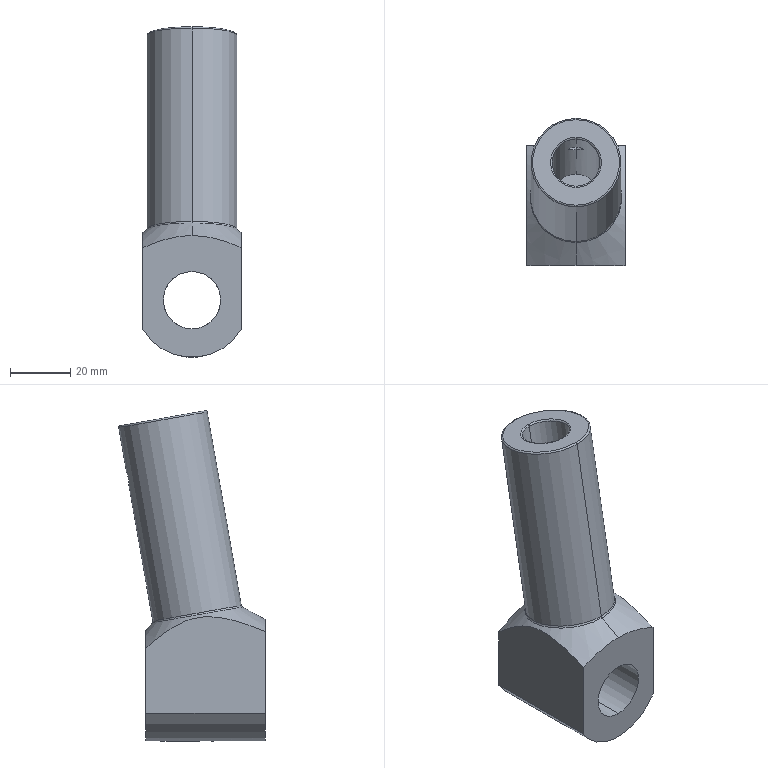Part | SolidWorks | features ICE 6, Fillet 2, 3DProfileFeature 1, Extrusion 1, HoleWzd 1, RevCutThin 1 | 1 solid | 27 faces | box 32.614 x 48.684 x 109.683 mm | volume 70811 mm3 | cylinder 12 | plane 7 | torus 6 | cone 2 | commonest cylinder face diameters 4.762 x2 5.41 x2 15.888 x2 19.05 x2 29.845 x2 15.875 x1
STEP:
#1=CARTESIAN_POINT('',(0.,1.053,2.59));
#2=VERTEX_POINT('',#1);
#3=CARTESIAN_POINT('',(0.,1.086,2.774));
#4=VERTEX_POINT('',#3);
#5=CARTESIAN_POINT('',(0.,1.053,2.59));
#6=CARTESIAN_POINT('',(-0.006205,1.053,2.59));
#7=CARTESIAN_POINT('',(-0.0123,1.053,2.59));
#8=CARTESIAN_POINT('',(-0.0243,1.053,2.593));
#9=CARTESIAN_POINT('',(-0.03026,1.053,2.595));
#10=CARTESIAN_POINT('',(-0.04161,1.053,2.599));
#11=CARTESIAN_POINT('',(-0.04699,1.054,2.602));
#12=CARTESIAN_POINT('',(-0.05718,1.054,2.609));
#13=CARTESIAN_POINT('',(-0.06199,1.054,2.613));
#14=CARTESIAN_POINT('',(-0.07494,1.055,2.626));
#15=CARTESIAN_POINT('',(-0.08192,1.056,2.637));
#16=CARTESIAN_POINT('',(-0.08894,1.058,2.653));
#17=CARTESIAN_POINT('',(-0.09074,1.058,2.659));
#18=CARTESIAN_POINT('',(-0.09315,1.06,2.671));
#19=CARTESIAN_POINT('',(-0.09375,1.061,2.677));
#20=CARTESIAN_POINT('',(-0.09375,1.063,2.689));
#21=CARTESIAN_POINT('',(-0.09314,1.064,2.696));
#22=CARTESIAN_POINT('',(-0.09074,1.067,2.707));
#23=CARTESIAN_POINT('',(-0.08897,1.068,2.713));
#24=CARTESIAN_POINT('',(-0.08426,1.071,2.724));
#25=CARTESIAN_POINT('',(-0.08133,1.072,2.729));
#26=CARTESIAN_POINT('',(-0.07454,1.075,2.739));
#27=CARTESIAN_POINT('',(-0.07066,1.076,2.744));
#28=CARTESIAN_POINT('',(-0.06193,1.079,2.752));
#29=CARTESIAN_POINT('',(-0.0572,1.08,2.756));
#30=CARTESIAN_POINT('',(-0.04706,1.082,2.763));
#31=CARTESIAN_POINT('',(-0.04157,1.083,2.765));
#32=CARTESIAN_POINT('',(-0.03023,1.084,2.77));
#33=CARTESIAN_POINT('',(-0.02438,1.085,2.772));
#34=CARTESIAN_POINT('',(-0.01234,1.086,2.774));
#35=CARTESIAN_POINT('',(-0.006124,1.086,2.774));
#36=CARTESIAN_POINT('',(0.,1.086,2.774));
#37=B_SPLINE_CURVE_WITH_KNOTS('',3,(#5,#6,#7,#8,#9,#10,#11,#12,#13,#14,#15,#16,#17,#18,#19,#20,#21,#22,#23,#24,#25,#26,#27,#28,#29,#30,#31,#32,#33,#34,#35,#36),.UNSPECIFIED.,.F.,.F.,(4,2,2,2,2,2,2,2,2,2,2,2,2,2,2,4),(0.,0.000466,0.0009321,0.001398,0.001864,0.002796,0.003262,0.003728,0.004194,0.00466,0.005127,0.005593,0.006059,0.006525,0.006991,0.007457),.UNSPECIFIED.);
#38=EDGE_CURVE('',#2,#4,#37,.T.);
#39=ORIENTED_EDGE('',*,*,#38,.T.);
#40=CARTESIAN_POINT('',(0.,0.8152,2.822));
#41=VERTEX_POINT('',#40);
#42=CARTESIAN_POINT('',(0.,3.094,2.42));
#43=DIRECTION('',(0.,-0.9848,0.1736));
#44=VECTOR('',#43,39.37);
#45=LINE('',#42,#44);
#46=EDGE_CURVE('',#4,#41,#45,.T.);
#47=ORIENTED_EDGE('',*,*,#46,.T.);
#48=CARTESIAN_POINT('',(0.,0.7826,2.637));
#49=VERTEX_POINT('',#48);
#50=CARTESIAN_POINT('',(0.,0.7826,2.637));
#51=CARTESIAN_POINT('',(-0.006233,0.7826,2.637));
#52=CARTESIAN_POINT('',(-0.01235,0.7826,2.638));
#53=CARTESIAN_POINT('',(-0.02439,0.7823,2.641));
#54=CARTESIAN_POINT('',(-0.03036,0.7821,2.642));
#55=CARTESIAN_POINT('',(-0.0417,0.7816,2.647));
#56=CARTESIAN_POINT('',(-0.04707,0.7813,2.65));
#57=CARTESIAN_POINT('',(-0.05724,0.7808,2.657));
#58=CARTESIAN_POINT('',(-0.06202,0.7806,2.661));
#59=CARTESIAN_POINT('',(-0.07491,0.7801,2.675));
#60=CARTESIAN_POINT('',(-0.08188,0.78,2.685));
#61=CARTESIAN_POINT('',(-0.0889,0.7809,2.702));
#62=CARTESIAN_POINT('',(-0.09072,0.7814,2.708));
#63=CARTESIAN_POINT('',(-0.09314,0.7828,2.72));
#64=CARTESIAN_POINT('',(-0.09375,0.7837,2.726));
#65=CARTESIAN_POINT('',(-0.09375,0.7858,2.738));
#66=CARTESIAN_POINT('',(-0.09313,0.7871,2.744));
#67=CARTESIAN_POINT('',(-0.09072,0.7899,2.756));
#68=CARTESIAN_POINT('',(-0.08894,0.7915,2.762));
#69=CARTESIAN_POINT('',(-0.08183,0.7964,2.778));
#70=CARTESIAN_POINT('',(-0.07493,0.8001,2.788));
#71=CARTESIAN_POINT('',(-0.06194,0.8051,2.8));
#72=CARTESIAN_POINT('',(-0.05725,0.8067,2.804));
#73=CARTESIAN_POINT('',(-0.04711,0.8096,2.81));
#74=CARTESIAN_POINT('',(-0.04162,0.8109,2.813));
#75=CARTESIAN_POINT('',(-0.03032,0.813,2.818));
#76=CARTESIAN_POINT('',(-0.02447,0.8138,2.819));
#77=CARTESIAN_POINT('',(-0.01236,0.8149,2.822));
#78=CARTESIAN_POINT('',(-0.006142,0.8152,2.822));
#79=CARTESIAN_POINT('',(0.,0.8152,2.822));
#80=B_SPLINE_CURVE_WITH_KNOTS('',3,(#50,#51,#52,#53,#54,#55,#56,#57,#58,#59,#60,#61,#62,#63,#64,#65,#66,#67,#68,#69,#70,#71,#72,#73,#74,#75,#76,#77,#78,#79),.UNSPECIFIED.,.F.,.F.,(4,2,2,2,2,2,2,2,2,2,2,2,2,2,4),(0.,0.000468,0.000936,0.001404,0.001872,0.002808,0.003276,0.003744,0.004212,0.00468,0.005616,0.006084,0.006552,0.00702,0.007488),.UNSPECIFIED.);
#81=EDGE_CURVE('',#49,#41,#80,.T.);
#82=ORIENTED_EDGE('',*,*,#81,.F.);
#83=CARTESIAN_POINT('',(0.,3.062,2.236));
#84=DIRECTION('',(0.,-0.9848,0.1736));
#85=VECTOR('',#84,39.37);
#86=LINE('',#83,#85);
#87=EDGE_CURVE('',#2,#49,#86,.T.);
#88=ORIENTED_EDGE('',*,*,#87,.F.);
#89=EDGE_LOOP('',(#39,#47,#82,#88));
#90=FACE_OUTER_BOUND('',#89,.T.);
#91=CARTESIAN_POINT('',(0.,3.078,2.328));
#92=DIRECTION('',(0.,-0.9848,0.1736));
#93=DIRECTION('',(0.,-0.1736,-0.9848));
#94=AXIS2_PLACEMENT_3D('',#91,#92,#93);
#95=CYLINDRICAL_SURFACE('',#94,0.09375);
#96=ADVANCED_FACE('',(#90),#95,.F.);
#97=CARTESIAN_POINT('',(0.1065,0.05244,-0.3596));
#98=VERTEX_POINT('',#97);
#99=CARTESIAN_POINT('',(0.,-0.05406,-0.375));
#100=VERTEX_POINT('',#99);
#101=CARTESIAN_POINT('',(0.1065,0.05244,-0.3596));
#102=CARTESIAN_POINT('',(0.1065,0.0385,-0.3596));
#103=CARTESIAN_POINT('',(0.1037,0.02442,-0.3604));
#104=CARTESIAN_POINT('',(0.09569,0.005169,-0.3626));
#105=CARTESIAN_POINT('',(0.09235,-0.001061,-0.3635));
#106=CARTESIAN_POINT('',(0.08462,-0.01259,-0.3653));
#107=CARTESIAN_POINT('',(0.08024,-0.01793,-0.3663));
#108=CARTESIAN_POINT('',(0.07042,-0.02776,-0.3684));
#109=CARTESIAN_POINT('',(0.06499,-0.03222,-0.3694));
#110=CARTESIAN_POINT('',(0.0535,-0.03991,-0.3712));
#111=CARTESIAN_POINT('',(0.04739,-0.04319,-0.3721));
#112=CARTESIAN_POINT('',(0.0344,-0.04859,-0.3735));
#113=CARTESIAN_POINT('',(0.02773,-0.05062,-0.374));
#114=CARTESIAN_POINT('',(0.01408,-0.05335,-0.3748));
#115=CARTESIAN_POINT('',(0.007021,-0.05406,-0.375));
#116=CARTESIAN_POINT('',(0.,-0.05406,-0.375));
#117=B_SPLINE_CURVE_WITH_KNOTS('',3,(#101,#102,#103,#104,#105,#106,#107,#108,#109,#110,#111,#112,#113,#114,#115,#116),.UNSPECIFIED.,.F.,.F.,(4,2,2,2,2,2,2,4),(0.008501,0.009564,0.01009,0.01063,0.01116,0.01169,0.01222,0.01275),.UNSPECIFIED.);
#118=EDGE_CURVE('',#98,#100,#117,.T.);
#119=ORIENTED_EDGE('',*,*,#118,.F.);
#120=CARTESIAN_POINT('',(0.1065,0.05244,-0.7383));
#121=VERTEX_POINT('',#120);
#122=CARTESIAN_POINT('',(0.1065,0.05244,-0.7459));
#123=DIRECTION('',(0.,0.,-1.));
#124=VECTOR('',#123,39.37);
#125=LINE('',#122,#124);
#126=EDGE_CURVE('',#98,#121,#125,.T.);
#127=ORIENTED_EDGE('',*,*,#126,.T.);
#128=CARTESIAN_POINT('',(-0.1065,0.05244,-0.7383));
#129=VERTEX_POINT('',#128);
#130=CARTESIAN_POINT('',(-0.1065,0.05244,-0.7383));
#131=CARTESIAN_POINT('',(-0.1065,0.0454,-0.7383));
#132=CARTESIAN_POINT('',(-0.1058,0.03847,-0.7384));
#133=CARTESIAN_POINT('',(-0.1031,0.02484,-0.7387));
#134=CARTESIAN_POINT('',(-0.101,0.01807,-0.739));
#135=CARTESIAN_POINT('',(-0.09569,0.00518,-0.7397));
#136=CARTESIAN_POINT('',(-0.09242,-0.0009336,-0.7402));
#137=CARTESIAN_POINT('',(-0.08469,-0.0125,-0.7411));
#138=CARTESIAN_POINT('',(-0.0802,-0.01798,-0.7416));
#139=CARTESIAN_POINT('',(-0.07038,-0.02779,-0.7426));
#140=CARTESIAN_POINT('',(-0.06503,-0.03219,-0.7431));
#141=CARTESIAN_POINT('',(-0.05339,-0.03998,-0.744));
#142=CARTESIAN_POINT('',(-0.0472,-0.04328,-0.7444));
#143=CARTESIAN_POINT('',(-0.03439,-0.04859,-0.7451));
#144=CARTESIAN_POINT('',(-0.02767,-0.05064,-0.7454));
#145=CARTESIAN_POINT('',(-0.01391,-0.05338,-0.7458));
#146=CARTESIAN_POINT('',(-0.006996,-0.05406,-0.7459));
#147=CARTESIAN_POINT('',(0.006917,-0.05406,-0.7459));
#148=CARTESIAN_POINT('',(0.01398,-0.05337,-0.7458));
#149=CARTESIAN_POINT('',(0.02765,-0.05064,-0.7454));
#150=CARTESIAN_POINT('',(0.03429,-0.04863,-0.7451));
#151=CARTESIAN_POINT('',(0.0472,-0.04328,-0.7444));
#152=CARTESIAN_POINT('',(0.05342,-0.03995,-0.744));
#153=CARTESIAN_POINT('',(0.06495,-0.03224,-0.7431));
#154=CARTESIAN_POINT('',(0.07034,-0.02783,-0.7426));
#155=CARTESIAN_POINT('',(0.08027,-0.01791,-0.7416));
#156=CARTESIAN_POINT('',(0.08467,-0.01253,-0.7411));
#157=CARTESIAN_POINT('',(0.09238,-0.001008,-0.7402));
#158=CARTESIAN_POINT('',(0.09572,0.005224,-0.7397));
#159=CARTESIAN_POINT('',(0.1011,0.01811,-0.739));
#160=CARTESIAN_POINT('',(0.1031,0.02475,-0.7387));
#161=CARTESIAN_POINT('',(0.1058,0.03842,-0.7384));
#162=CARTESIAN_POINT('',(0.1065,0.04549,-0.7383));
#163=CARTESIAN_POINT('',(0.1065,0.05244,-0.7383));
#164=B_SPLINE_CURVE_WITH_KNOTS('',3,(#130,#131,#132,#133,#134,#135,#136,#137,#138,#139,#140,#141,#142,#143,#144,#145,#146,#147,#148,#149,#150,#151,#152,#153,#154,#155,#156,#157,#158,#159,#160,#161,#162,#163),.UNSPECIFIED.,.F.,.F.,(4,2,2,2,2,2,2,2,2,2,2,2,2,2,2,2,4),(0.,0.0005293,0.001059,0.001588,0.002117,0.002646,0.003176,0.003705,0.004234,0.004763,0.005293,0.005822,0.006351,0.00688,0.00741,0.007939,0.008468),.UNSPECIFIED.);
#165=EDGE_CURVE('',#129,#121,#164,.T.);
#166=ORIENTED_EDGE('',*,*,#165,.F.);
#167=CARTESIAN_POINT('',(-0.1065,0.05244,-0.3596));
#168=VERTEX_POINT('',#167);
#169=CARTESIAN_POINT('',(-0.1065,0.05244,-0.7459));
#170=DIRECTION('',(0.,0.,-1.));
#171=VECTOR('',#170,39.37);
#172=LINE('',#169,#171);
#173=EDGE_CURVE('',#168,#129,#172,.T.);
#174=ORIENTED_EDGE('',*,*,#173,.F.);
#175=CARTESIAN_POINT('',(0.,-0.05406,-0.375));
#176=CARTESIAN_POINT('',(-0.00702,-0.05406,-0.375));
#177=CARTESIAN_POINT('',(-0.01396,-0.05337,-0.3748));
#178=CARTESIAN_POINT('',(-0.02766,-0.05064,-0.374));
#179=CARTESIAN_POINT('',(-0.03446,-0.04857,-0.3735));
#180=CARTESIAN_POINT('',(-0.05371,-0.04057,-0.3714));
#181=CARTESIAN_POINT('',(-0.06552,-0.03265,-0.3694));
#182=CARTESIAN_POINT('',(-0.08017,-0.018,-0.3664));
#183=CARTESIAN_POINT('',(-0.08463,-0.01258,-0.3653));
#184=CARTESIAN_POINT('',(-0.09237,-0.00102,-0.3635));
#185=CARTESIAN_POINT('',(-0.09564,0.005076,-0.3626));
#186=CARTESIAN_POINT('',(-0.101,0.01791,-0.3612));
#187=CARTESIAN_POINT('',(-0.1031,0.0247,-0.3606));
#188=CARTESIAN_POINT('',(-0.1058,0.03841,-0.3598));
#189=CARTESIAN_POINT('',(-0.1065,0.04537,-0.3596));
#190=CARTESIAN_POINT('',(-0.1065,0.05244,-0.3596));
#191=B_SPLINE_CURVE_WITH_KNOTS('',3,(#175,#176,#177,#178,#179,#180,#181,#182,#183,#184,#185,#186,#187,#188,#189,#190),.UNSPECIFIED.,.F.,.F.,(4,2,2,2,2,2,2,4),(0.01275,0.01328,0.01381,0.01488,0.01541,0.01594,0.01647,0.017),.UNSPECIFIED.);
#192=EDGE_CURVE('',#100,#168,#191,.T.);
#193=ORIENTED_EDGE('',*,*,#192,.F.);
#194=EDGE_LOOP('',(#119,#127,#166,#174,#193));
#195=FACE_OUTER_BOUND('',#194,.T.);
#196=CARTESIAN_POINT('',(0.,0.05244,-0.7459));
#197=DIRECTION('',(0.,0.,-1.));
#198=DIRECTION('',(-1.,0.,0.));
#199=AXIS2_PLACEMENT_3D('',#196,#197,#198);
#200=CYLINDRICAL_SURFACE('',#199,0.1065);
#201=ADVANCED_FACE('',(#195),#200,.F.);
#202=CARTESIAN_POINT('',(0.,0.301,3.508));
#203=VERTEX_POINT('',#202);
#204=CARTESIAN_POINT('',(0.,0.917,3.399));
#205=VERTEX_POINT('',#204);
#206=CARTESIAN_POINT('',(0.,0.609,3.454));
#207=DIRECTION('',(0.,0.1736,0.9848));
#208=DIRECTION('',(0.,0.9848,-0.1736));
#209=AXIS2_PLACEMENT_3D('',#206,#207,#208);
#210=CIRCLE('',#209,0.3128);
#211=EDGE_CURVE('',#203,#205,#210,.T.);
#212=ORIENTED_EDGE('',*,*,#211,.F.);
#213=CARTESIAN_POINT('',(0.,0.2848,3.531));
#214=VERTEX_POINT('',#213);
#215=CARTESIAN_POINT('',(0.,0.2813,3.512));
#216=DIRECTION('',(1.,0.,0.));
#217=DIRECTION('',(0.,1.,0.));
#218=AXIS2_PLACEMENT_3D('',#215,#216,#217);
#219=CIRCLE('',#218,0.02);
#220=EDGE_CURVE('',#203,#214,#219,.T.);
#221=ORIENTED_EDGE('',*,*,#220,.T.);
#222=CARTESIAN_POINT('',(0.,0.9402,3.416));
#223=VERTEX_POINT('',#222);
#224=CARTESIAN_POINT('',(0.,0.6125,3.473));
#225=DIRECTION('',(0.,-0.1736,-0.9848));
#226=DIRECTION('',(0.,0.9848,-0.1736));
#227=AXIS2_PLACEMENT_3D('',#224,#225,#226);
#228=CIRCLE('',#227,0.3327);
#229=EDGE_CURVE('',#223,#214,#228,.T.);
#230=ORIENTED_EDGE('',*,*,#229,.F.);
#231=CARTESIAN_POINT('',(0.,0.9367,3.396));
#232=DIRECTION('',(-1.,0.,0.));
#233=DIRECTION('',(0.,0.,1.));
#234=AXIS2_PLACEMENT_3D('',#231,#232,#233);
#235=CIRCLE('',#234,0.02);
#236=EDGE_CURVE('',#205,#223,#235,.T.);
#237=ORIENTED_EDGE('',*,*,#236,.F.);
#238=EDGE_LOOP('',(#212,#221,#230,#237));
#239=FACE_OUTER_BOUND('',#238,.T.);
#240=CARTESIAN_POINT('',(0.,0.609,3.454));
#241=DIRECTION('',(0.,-0.1736,-0.9848));
#242=DIRECTION('',(0.,0.9848,-0.1736));
#243=AXIS2_PLACEMENT_3D('',#240,#241,#242);
#244=TOROIDAL_SURFACE('',#243,0.3327,0.02);
#245=ADVANCED_FACE('',(#239),#244,.T.);
#246=CARTESIAN_POINT('',(0.,0.05359,3.572));
#247=VERTEX_POINT('',#246);
#248=CARTESIAN_POINT('',(0.,1.171,3.375));
#249=VERTEX_POINT('',#248);
#250=CARTESIAN_POINT('',(0.,0.6125,3.473));
#251=DIRECTION('',(0.,0.1736,0.9848));
#252=DIRECTION('',(0.,0.9848,-0.1736));
#253=AXIS2_PLACEMENT_3D('',#250,#251,#252);
#254=CIRCLE('',#253,0.5675);
#255=EDGE_CURVE('',#247,#249,#254,.T.);
#256=ORIENTED_EDGE('',*,*,#255,.F.);
#257=CARTESIAN_POINT('',(0.,0.03042,3.556));
#258=VERTEX_POINT('',#257);
#259=CARTESIAN_POINT('',(0.,0.05012,3.552));
#260=DIRECTION('',(1.,0.,0.));
#261=DIRECTION('',(0.,1.,0.));
#262=AXIS2_PLACEMENT_3D('',#259,#260,#261);
#263=CIRCLE('',#262,0.02);
#264=EDGE_CURVE('',#247,#258,#263,.T.);
#265=ORIENTED_EDGE('',*,*,#264,.T.);
#266=CARTESIAN_POINT('',(0.,1.188,3.352));
#267=VERTEX_POINT('',#266);
#268=CARTESIAN_POINT('',(0.,0.609,3.454));
#269=DIRECTION('',(0.,-0.1736,-0.9848));
#270=DIRECTION('',(0.,0.9848,-0.1736));
#271=AXIS2_PLACEMENT_3D('',#268,#269,#270);
#272=CIRCLE('',#271,0.5875);
#273=EDGE_CURVE('',#267,#258,#272,.T.);
#274=ORIENTED_EDGE('',*,*,#273,.F.);
#275=CARTESIAN_POINT('',(0.,1.168,3.355));
#276=DIRECTION('',(-1.,0.,0.));
#277=DIRECTION('',(0.,0.,1.));
#278=AXIS2_PLACEMENT_3D('',#275,#276,#277);
#279=CIRCLE('',#278,0.02);
#280=EDGE_CURVE('',#249,#267,#279,.T.);
#281=ORIENTED_EDGE('',*,*,#280,.F.);
#282=EDGE_LOOP('',(#256,#265,#274,#281));
#283=FACE_OUTER_BOUND('',#282,.T.);
#284=CARTESIAN_POINT('',(0.,0.609,3.454));
#285=DIRECTION('',(0.,-0.1736,-0.9848));
#286=DIRECTION('',(0.,0.9848,-0.1736));
#287=AXIS2_PLACEMENT_3D('',#284,#285,#286);
#288=TOROIDAL_SURFACE('',#287,0.5675,0.02);
#289=ADVANCED_FACE('',(#283),#288,.T.);
#290=CARTESIAN_POINT('',(0.,0.742,0.825));
#291=VERTEX_POINT('',#290);
#292=CARTESIAN_POINT('',(0.,-0.4151,1.029));
#293=VERTEX_POINT('',#292);
#294=CARTESIAN_POINT('',(0.,0.1635,0.9271));
#295=DIRECTION('',(0.,0.1736,0.9848));
#296=DIRECTION('',(0.,-0.9848,0.1736));
#297=AXIS2_PLACEMENT_3D('',#294,#295,#296);
#298=CIRCLE('',#297,0.5875);
#299=EDGE_CURVE('',#291,#293,#298,.T.);
#300=ORIENTED_EDGE('',*,*,#299,.F.);
#301=CARTESIAN_POINT('',(0.,0.7489,0.8002));
#302=VERTEX_POINT('',#301);
#303=CARTESIAN_POINT('',(0.,0.7716,0.8198));
#304=DIRECTION('',(1.,0.,0.));
#305=DIRECTION('',(0.,1.,0.));
#306=AXIS2_PLACEMENT_3D('',#303,#304,#305);
#307=CIRCLE('',#306,0.03);
#308=EDGE_CURVE('',#291,#302,#307,.T.);
#309=ORIENTED_EDGE('',*,*,#308,.T.);
#310=CARTESIAN_POINT('',(0.,-0.4301,1.008));
#311=VERTEX_POINT('',#310);
#312=CARTESIAN_POINT('',(0.,0.1594,0.9041));
#313=DIRECTION('',(0.,-0.1736,-0.9848));
#314=DIRECTION('',(0.,0.9848,-0.1736));
#315=AXIS2_PLACEMENT_3D('',#312,#313,#314);
#316=CIRCLE('',#315,0.5986);
#317=EDGE_CURVE('',#311,#302,#316,.T.);
#318=ORIENTED_EDGE('',*,*,#317,.F.);
#319=CARTESIAN_POINT('',(0.,-0.4447,1.034));
#320=DIRECTION('',(-1.,0.,0.));
#321=DIRECTION('',(0.,0.,1.));
#322=AXIS2_PLACEMENT_3D('',#319,#320,#321);
#323=CIRCLE('',#322,0.03);
#324=EDGE_CURVE('',#293,#311,#323,.T.);
#325=ORIENTED_EDGE('',*,*,#324,.F.);
#326=EDGE_LOOP('',(#300,#309,#318,#325));
#327=FACE_OUTER_BOUND('',#326,.T.);
#328=CARTESIAN_POINT('',(0.,0.1635,0.9271));
#329=DIRECTION('',(0.,0.1736,0.9848));
#330=DIRECTION('',(0.,-0.9848,0.1736));
#331=AXIS2_PLACEMENT_3D('',#328,#329,#330);
#332=TOROIDAL_SURFACE('',#331,0.6175,0.03);
#333=ADVANCED_FACE('',(#327),#332,.F.);
#334=CARTESIAN_POINT('',(0.,-0.7288,-0.375));
#335=VERTEX_POINT('',#334);
#336=CARTESIAN_POINT('',(0.,-0.7288,0.375));
#337=VERTEX_POINT('',#336);
#338=CARTESIAN_POINT('',(0.,-0.7288,0.));
#339=DIRECTION('',(0.,1.,0.));
#340=DIRECTION('',(0.,0.,1.));
#341=AXIS2_PLACEMENT_3D('',#338,#339,#340);
#342=CIRCLE('',#341,0.375);
#343=EDGE_CURVE('',#335,#337,#342,.T.);
#344=ORIENTED_EDGE('',*,*,#343,.F.);
#345=CARTESIAN_POINT('',(0.,-0.7288,-0.375));
#346=DIRECTION('',(0.,1.,0.));
#347=VECTOR('',#346,39.37);
#348=LINE('',#345,#347);
#349=EDGE_CURVE('',#335,#100,#348,.T.);
#350=ORIENTED_EDGE('',*,*,#349,.T.);
#351=ORIENTED_EDGE('',*,*,#192,.T.);
#352=CARTESIAN_POINT('',(0.,0.1589,-0.375));
#353=VERTEX_POINT('',#352);
#354=CARTESIAN_POINT('',(-0.1065,0.05244,-0.3596));
#355=CARTESIAN_POINT('',(-0.1065,0.05952,-0.3596));
#356=CARTESIAN_POINT('',(-0.1058,0.06647,-0.3598));
#357=CARTESIAN_POINT('',(-0.1031,0.08014,-0.3606));
#358=CARTESIAN_POINT('',(-0.101,0.08692,-0.3612));
#359=CARTESIAN_POINT('',(-0.09564,0.0998,-0.3626));
#360=CARTESIAN_POINT('',(-0.09237,0.1059,-0.3635));
#361=CARTESIAN_POINT('',(-0.08464,0.1175,-0.3653));
#362=CARTESIAN_POINT('',(-0.08016,0.1229,-0.3664));
#363=CARTESIAN_POINT('',(-0.0655,0.1375,-0.3694));
#364=CARTESIAN_POINT('',(-0.05367,0.1455,-0.3714));
#365=CARTESIAN_POINT('',(-0.03446,0.1535,-0.3735));
#366=CARTESIAN_POINT('',(-0.0277,0.1555,-0.374));
#367=CARTESIAN_POINT('',(-0.01393,0.1583,-0.3748));
#368=CARTESIAN_POINT('',(-0.00699,0.1589,-0.375));
#369=CARTESIAN_POINT('',(0.,0.1589,-0.375));
#370=B_SPLINE_CURVE_WITH_KNOTS('',3,(#354,#355,#356,#357,#358,#359,#360,#361,#362,#363,#364,#365,#366,#367,#368,#369),.UNSPECIFIED.,.F.,.F.,(4,2,2,2,2,2,2,4),(0.,0.0005315,0.001063,0.001594,0.002126,0.003189,0.00372,0.004252),.UNSPECIFIED.);
#371=EDGE_CURVE('',#168,#353,#370,.T.);
#372=ORIENTED_EDGE('',*,*,#371,.T.);
#373=CARTESIAN_POINT('',(0.,0.6162,-0.375));
#374=VERTEX_POINT('',#373);
#375=CARTESIAN_POINT('',(0.,-0.7288,-0.375));
#376=DIRECTION('',(0.,1.,0.));
#377=VECTOR('',#376,39.37);
#378=LINE('',#375,#377);
#379=EDGE_CURVE('',#353,#374,#378,.T.);
#380=ORIENTED_EDGE('',*,*,#379,.T.);
#381=CARTESIAN_POINT('',(-0.3118,0.6162,-0.2083));
#382=VERTEX_POINT('',#381);
#383=CARTESIAN_POINT('',(0.,0.6162,0.));
#384=DIRECTION('',(0.,-1.,0.));
#385=DIRECTION('',(0.,0.,1.));
#386=AXIS2_PLACEMENT_3D('',#383,#384,#385);
#387=CIRCLE('',#386,0.375);
#388=EDGE_CURVE('',#382,#374,#387,.T.);
#389=ORIENTED_EDGE('',*,*,#388,.F.);
#390=CARTESIAN_POINT('',(-0.3118,0.8337,-0.2083));
#391=VERTEX_POINT('',#390);
#392=CARTESIAN_POINT('',(-0.3118,0.6162,-0.2083));
#393=DIRECTION('',(0.,1.,0.));
#394=VECTOR('',#393,39.37);
#395=LINE('',#392,#394);
#396=EDGE_CURVE('',#382,#391,#395,.T.);
#397=ORIENTED_EDGE('',*,*,#396,.T.);
#398=CARTESIAN_POINT('',(0.,0.8337,0.375));
#399=VERTEX_POINT('',#398);
#400=CARTESIAN_POINT('',(0.,0.8337,0.));
#401=DIRECTION('',(0.,-1.,0.));
#402=DIRECTION('',(0.,0.,-1.));
#403=AXIS2_PLACEMENT_3D('',#400,#401,#402);
#404=CIRCLE('',#403,0.375);
#405=EDGE_CURVE('',#399,#391,#404,.T.);
#406=ORIENTED_EDGE('',*,*,#405,.F.);
#407=CARTESIAN_POINT('',(0.,-0.7288,0.375));
#408=DIRECTION('',(0.,1.,0.));
#409=VECTOR('',#408,39.37);
#410=LINE('',#407,#409);
#411=EDGE_CURVE('',#337,#399,#410,.T.);
#412=ORIENTED_EDGE('',*,*,#411,.F.);
#413=EDGE_LOOP('',(#344,#350,#351,#372,#380,#389,#397,#406,#412));
#414=FACE_OUTER_BOUND('',#413,.T.);
#415=CARTESIAN_POINT('',(0.,-0.7288,0.));
#416=DIRECTION('',(0.,1.,0.));
#417=DIRECTION('',(0.,0.,1.));
#418=AXIS2_PLACEMENT_3D('',#415,#416,#417);
#419=CYLINDRICAL_SURFACE('',#418,0.375);
#420=ADVANCED_FACE('',(#414),#419,.F.);
#421=CARTESIAN_POINT('',(0.,0.1594,0.9041));
#422=DIRECTION('',(0.,-0.1736,-0.9848));
#423=DIRECTION('',(0.,0.9848,-0.1736));
#424=AXIS2_PLACEMENT_3D('',#421,#422,#423);
#425=CIRCLE('',#424,0.5986);
#426=EDGE_CURVE('',#302,#311,#425,.T.);
#427=ORIENTED_EDGE('',*,*,#426,.T.);
#428=CARTESIAN_POINT('',(0.,-0.7288,0.842));
#429=VERTEX_POINT('',#428);
#430=CARTESIAN_POINT('',(0.,-0.4176,1.015));
#431=DIRECTION('',(0.,-0.874,-0.4859));
#432=VECTOR('',#431,39.37);
#433=LINE('',#430,#432);
#434=EDGE_CURVE('',#311,#429,#433,.T.);
#435=ORIENTED_EDGE('',*,*,#434,.T.);
#436=CARTESIAN_POINT('',(0.642,-0.7288,0.6849));
#437=VERTEX_POINT('',#436);
#438=CARTESIAN_POINT('',(0.,-0.7288,0.842));
#439=CARTESIAN_POINT('',(0.02767,-0.7288,0.842));
#440=CARTESIAN_POINT('',(0.05544,-0.7288,0.841));
#441=CARTESIAN_POINT('',(0.1111,-0.7288,0.8372));
#442=CARTESIAN_POINT('',(0.139,-0.7288,0.8343));
#443=CARTESIAN_POINT('',(0.2216,-0.7288,0.823));
#444=CARTESIAN_POINT('',(0.2758,-0.7288,0.8119));
#445=CARTESIAN_POINT('',(0.3828,-0.7288,0.7839));
#446=CARTESIAN_POINT('',(0.4357,-0.7288,0.7671));
#447=CARTESIAN_POINT('',(0.5141,-0.7288,0.7384));
#448=CARTESIAN_POINT('',(0.5401,-0.7288,0.7283));
#449=CARTESIAN_POINT('',(0.5914,-0.7288,0.7072));
#450=CARTESIAN_POINT('',(0.6168,-0.7288,0.6962));
#451=CARTESIAN_POINT('',(0.642,-0.7288,0.6849));
#452=B_SPLINE_CURVE_WITH_KNOTS('',3,(#438,#439,#440,#441,#442,#443,#444,#445,#446,#447,#448,#449,#450,#451),.UNSPECIFIED.,.F.,.F.,(4,2,2,2,2,2,4),(0.06577,0.06786,0.06995,0.07413,0.07831,0.0804,0.08249),.UNSPECIFIED.);
#453=EDGE_CURVE('',#429,#437,#452,.T.);
#454=ORIENTED_EDGE('',*,*,#453,.T.);
#455=CARTESIAN_POINT('',(0.642,0.8337,0.4716));
#456=VERTEX_POINT('',#455);
#457=CARTESIAN_POINT('',(0.642,0.8337,0.4716));
#458=CARTESIAN_POINT('',(0.642,0.7803,0.5189));
#459=CARTESIAN_POINT('',(0.642,0.7258,0.5649));
#460=CARTESIAN_POINT('',(0.642,0.6412,0.6308));
#461=CARTESIAN_POINT('',(0.642,0.6125,0.6523));
#462=CARTESIAN_POINT('',(0.642,0.554,0.6936));
#463=CARTESIAN_POINT('',(0.642,0.5243,0.7134));
#464=CARTESIAN_POINT('',(0.642,0.4333,0.7695));
#465=CARTESIAN_POINT('',(0.642,0.3701,0.8025));
#466=CARTESIAN_POINT('',(0.642,0.2691,0.8407));
#467=CARTESIAN_POINT('',(0.642,0.2349,0.8514));
#468=CARTESIAN_POINT('',(0.642,0.1658,0.8679));
#469=CARTESIAN_POINT('',(0.642,0.1307,0.8739));
#470=CARTESIAN_POINT('',(0.642,0.07757,0.8792));
#471=CARTESIAN_POINT('',(0.642,0.05974,0.8805));
#472=CARTESIAN_POINT('',(0.642,0.02386,0.8818));
#473=CARTESIAN_POINT('',(0.642,0.0058,0.8818));
#474=CARTESIAN_POINT('',(0.642,-0.04795,0.8805));
#475=CARTESIAN_POINT('',(0.642,-0.08344,0.8775));
#476=CARTESIAN_POINT('',(0.642,-0.1891,0.8638));
#477=CARTESIAN_POINT('',(0.642,-0.2586,0.8484));
#478=CARTESIAN_POINT('',(0.642,-0.3618,0.8197));
#479=CARTESIAN_POINT('',(0.642,-0.3961,0.8092));
#480=CARTESIAN_POINT('',(0.642,-0.4639,0.787));
#481=CARTESIAN_POINT('',(0.642,-0.4974,0.7753));
#482=CARTESIAN_POINT('',(0.642,-0.5976,0.7386));
#483=CARTESIAN_POINT('',(0.642,-0.6634,0.7123));
#484=CARTESIAN_POINT('',(0.642,-0.7288,0.6849));
#485=B_SPLINE_CURVE_WITH_KNOTS('',3,(#457,#458,#459,#460,#461,#462,#463,#464,#465,#466,#467,#468,#469,#470,#471,#472,#473,#474,#475,#476,#477,#478,#479,#480,#481,#482,#483,#484),.UNSPECIFIED.,.F.,.F.,(4,2,2,2,2,2,2,2,2,2,2,2,2,4),(0.06804,0.07348,0.0762,0.07892,0.08436,0.08708,0.0898,0.09116,0.09252,0.09524,0.1007,0.1034,0.1061,0.1116),.UNSPECIFIED.);
#486=EDGE_CURVE('',#456,#437,#485,.T.);
#487=ORIENTED_EDGE('',*,*,#486,.F.);
#488=CARTESIAN_POINT('',(0.,0.8337,0.7024));
#489=VERTEX_POINT('',#488);
#490=CARTESIAN_POINT('',(0.642,0.8337,0.4716));
#491=CARTESIAN_POINT('',(0.5932,0.8337,0.5012));
#492=CARTESIAN_POINT('',(0.5438,0.8337,0.5296));
#493=CARTESIAN_POINT('',(0.4426,0.8337,0.5829));
#494=CARTESIAN_POINT('',(0.3909,0.8337,0.6077));
#495=CARTESIAN_POINT('',(0.3104,0.8337,0.6403));
#496=CARTESIAN_POINT('',(0.283,0.8337,0.6504));
#497=CARTESIAN_POINT('',(0.228,0.8337,0.6682));
#498=CARTESIAN_POINT('',(0.2002,0.8337,0.676));
#499=CARTESIAN_POINT('',(0.1441,0.8337,0.6888));
#500=CARTESIAN_POINT('',(0.1157,0.8337,0.6938));
#501=CARTESIAN_POINT('',(0.07266,0.8337,0.6989));
#502=CARTESIAN_POINT('',(0.05822,0.8337,0.7002));
#503=CARTESIAN_POINT('',(0.02914,0.8337,0.702));
#504=CARTESIAN_POINT('',(0.01451,0.8337,0.7024));
#505=CARTESIAN_POINT('',(0.,0.8337,0.7024));
#506=B_SPLINE_CURVE_WITH_KNOTS('',3,(#490,#491,#492,#493,#494,#495,#496,#497,#498,#499,#500,#501,#502,#503,#504,#505),.UNSPECIFIED.,.F.,.F.,(4,2,2,2,2,2,2,4),(0.04699,0.05135,0.05571,0.05789,0.06006,0.06224,0.06333,0.06442),.UNSPECIFIED.);
#507=EDGE_CURVE('',#456,#489,#506,.T.);
#508=ORIENTED_EDGE('',*,*,#507,.T.);
#509=CARTESIAN_POINT('',(0.,0.7396,0.811));
#510=DIRECTION('',(0.,0.6552,-0.7555));
#511=VECTOR('',#510,39.37);
#512=LINE('',#509,#511);
#513=EDGE_CURVE('',#302,#489,#512,.T.);
#514=ORIENTED_EDGE('',*,*,#513,.F.);
#515=EDGE_LOOP('',(#427,#435,#454,#487,#508,#514));
#516=FACE_OUTER_BOUND('',#515,.T.);
#517=CARTESIAN_POINT('',(0.,0.161,0.913));
#518=DIRECTION('',(0.,-0.1736,-0.9848));
#519=DIRECTION('',(0.,0.9848,-0.1736));
#520=AXIS2_PLACEMENT_3D('',#517,#518,#519);
#521=CONICAL_SURFACE('',#520,0.5875,0.8889);
#522=ADVANCED_FACE('',(#516),#521,.T.);
#523=CARTESIAN_POINT('',(0.,0.4643,0.8321));
#524=VERTEX_POINT('',#523);
#525=CARTESIAN_POINT('',(0.,-0.1517,0.9407));
#526=VERTEX_POINT('',#525);
#527=CARTESIAN_POINT('',(0.,0.1563,0.8864));
#528=DIRECTION('',(0.,0.1736,0.9848));
#529=DIRECTION('',(0.,-0.9848,0.1736));
#530=AXIS2_PLACEMENT_3D('',#527,#528,#529);
#531=CIRCLE('',#530,0.3127);
#532=EDGE_CURVE('',#524,#526,#531,.T.);
#533=ORIENTED_EDGE('',*,*,#532,.F.);
#534=CARTESIAN_POINT('',(0.,0.4643,0.8321));
#535=DIRECTION('',(0.,0.1736,0.9848));
#536=VECTOR('',#535,39.37);
#537=LINE('',#534,#536);
#538=EDGE_CURVE('',#524,#49,#537,.T.);
#539=ORIENTED_EDGE('',*,*,#538,.T.);
#540=ORIENTED_EDGE('',*,*,#81,.T.);
#541=CARTESIAN_POINT('',(0.,0.4643,0.8321));
#542=DIRECTION('',(0.,0.1736,0.9848));
#543=VECTOR('',#542,39.37);
#544=LINE('',#541,#543);
#545=EDGE_CURVE('',#41,#205,#544,.T.);
#546=ORIENTED_EDGE('',*,*,#545,.T.);
#547=CARTESIAN_POINT('',(0.,0.609,3.454));
#548=DIRECTION('',(0.,0.1736,0.9848));
#549=DIRECTION('',(0.,0.9848,-0.1736));
#550=AXIS2_PLACEMENT_3D('',#547,#548,#549);
#551=CIRCLE('',#550,0.3128);
#552=EDGE_CURVE('',#205,#203,#551,.T.);
#553=ORIENTED_EDGE('',*,*,#552,.T.);
#554=CARTESIAN_POINT('',(0.,-0.1517,0.9407));
#555=DIRECTION('',(0.,0.1736,0.9848));
#556=VECTOR('',#555,39.37);
#557=LINE('',#554,#556);
#558=EDGE_CURVE('',#526,#203,#557,.T.);
#559=ORIENTED_EDGE('',*,*,#558,.F.);
#560=EDGE_LOOP('',(#533,#539,#540,#546,#553,#559));
#561=FACE_OUTER_BOUND('',#560,.T.);
#562=CARTESIAN_POINT('',(0.,0.1563,0.8864));
#563=DIRECTION('',(0.,0.1736,0.9848));
#564=DIRECTION('',(0.,-0.9848,0.1736));
#565=AXIS2_PLACEMENT_3D('',#562,#563,#564);
#566=CYLINDRICAL_SURFACE('',#565,0.3127);
#567=ADVANCED_FACE('',(#561),#566,.F.);
#568=CARTESIAN_POINT('',(0.,0.1635,0.9271));
#569=DIRECTION('',(0.,0.1736,0.9848));
#570=DIRECTION('',(0.,-0.9848,0.1736));
#571=AXIS2_PLACEMENT_3D('',#568,#569,#570);
#572=CIRCLE('',#571,0.5875);
#573=EDGE_CURVE('',#293,#291,#572,.T.);
#574=ORIENTED_EDGE('',*,*,#573,.T.);
#575=CARTESIAN_POINT('',(0.,0.7396,0.811));
#576=DIRECTION('',(0.,0.1736,0.9848));
#577=VECTOR('',#576,39.37);
#578=LINE('',#575,#577);
#579=EDGE_CURVE('',#291,#2,#578,.T.);
#580=ORIENTED_EDGE('',*,*,#579,.T.);
#581=CARTESIAN_POINT('',(0.,1.086,2.774));
#582=CARTESIAN_POINT('',(0.01224,1.086,2.774));
#583=CARTESIAN_POINT('',(0.0246,1.085,2.772));
#584=CARTESIAN_POINT('',(0.04152,1.083,2.765));
#585=CARTESIAN_POINT('',(0.04699,1.082,2.763));
#586=CARTESIAN_POINT('',(0.05721,1.08,2.756));
#587=CARTESIAN_POINT('',(0.06193,1.079,2.752));
#588=CARTESIAN_POINT('',(0.07057,1.076,2.744));
#589=CARTESIAN_POINT('',(0.07453,1.075,2.739));
#590=CARTESIAN_POINT('',(0.08133,1.072,2.729));
#591=CARTESIAN_POINT('',(0.08421,1.071,2.724));
#592=CARTESIAN_POINT('',(0.08893,1.068,2.713));
#593=CARTESIAN_POINT('',(0.09074,1.067,2.707));
#594=CARTESIAN_POINT('',(0.09313,1.064,2.696));
#595=CARTESIAN_POINT('',(0.09375,1.063,2.69));
#596=CARTESIAN_POINT('',(0.09375,1.061,2.677));
#597=CARTESIAN_POINT('',(0.09315,1.06,2.671));
#598=CARTESIAN_POINT('',(0.09077,1.058,2.659));
#599=CARTESIAN_POINT('',(0.08896,1.058,2.654));
#600=CARTESIAN_POINT('',(0.08427,1.056,2.642));
#601=CARTESIAN_POINT('',(0.08139,1.056,2.637));
#602=CARTESIAN_POINT('',(0.07459,1.055,2.627));
#603=CARTESIAN_POINT('',(0.07065,1.055,2.622));
#604=CARTESIAN_POINT('',(0.05771,1.054,2.609));
#605=CARTESIAN_POINT('',(0.04727,1.054,2.602));
#606=CARTESIAN_POINT('',(0.03037,1.053,2.595));
#607=CARTESIAN_POINT('',(0.02444,1.053,2.593));
#608=CARTESIAN_POINT('',(0.01233,1.053,2.59));
#609=CARTESIAN_POINT('',(0.006203,1.053,2.59));
#610=CARTESIAN_POINT('',(0.,1.053,2.59));
#611=B_SPLINE_CURVE_WITH_KNOTS('',3,(#581,#582,#583,#584,#585,#586,#587,#588,#589,#590,#591,#592,#593,#594,#595,#596,#597,#598,#599,#600,#601,#602,#603,#604,#605,#606,#607,#608,#609,#610),.UNSPECIFIED.,.F.,.F.,(4,2,2,2,2,2,2,2,2,2,2,2,2,2,4),(0.007457,0.008389,0.008855,0.009321,0.009786,0.01025,0.01072,0.01118,0.01165,0.01212,0.01258,0.01305,0.01398,0.01445,0.01491),.UNSPECIFIED.);
#612=EDGE_CURVE('',#4,#2,#611,.T.);
#613=ORIENTED_EDGE('',*,*,#612,.F.);
#614=CARTESIAN_POINT('',(0.,0.7396,0.811));
#615=DIRECTION('',(0.,0.1736,0.9848));
#616=VECTOR('',#615,39.37);
#617=LINE('',#614,#616);
#618=EDGE_CURVE('',#4,#267,#617,.T.);
#619=ORIENTED_EDGE('',*,*,#618,.T.);
#620=ORIENTED_EDGE('',*,*,#273,.T.);
#621=CARTESIAN_POINT('',(0.,-0.4176,1.015));
#622=DIRECTION('',(0.,0.1736,0.9848));
#623=VECTOR('',#622,39.37);
#624=LINE('',#621,#623);
#625=EDGE_CURVE('',#293,#258,#624,.T.);
#626=ORIENTED_EDGE('',*,*,#625,.F.);
#627=EDGE_LOOP('',(#574,#580,#613,#619,#620,#626));
#628=FACE_OUTER_BOUND('',#627,.T.);
#629=CARTESIAN_POINT('',(0.,0.161,0.913));
#630=DIRECTION('',(0.,0.1736,0.9848));
#631=DIRECTION('',(0.,-0.9848,0.1736));
#632=AXIS2_PLACEMENT_3D('',#629,#630,#631);
#633=CYLINDRICAL_SURFACE('',#632,0.5875);
#634=ADVANCED_FACE('',(#628),#633,.T.);
#635=CARTESIAN_POINT('',(0.,0.6125,3.473));
#636=DIRECTION('',(0.,0.1736,0.9848));
#637=DIRECTION('',(0.,0.9848,-0.1736));
#638=AXIS2_PLACEMENT_3D('',#635,#636,#637);
#639=CIRCLE('',#638,0.5675);
#640=EDGE_CURVE('',#249,#247,#639,.T.);
#641=ORIENTED_EDGE('',*,*,#640,.T.);
#642=ORIENTED_EDGE('',*,*,#255,.T.);
#643=EDGE_LOOP('',(#641,#642));
#644=FACE_OUTER_BOUND('',#643,.T.);
#645=ORIENTED_EDGE('',*,*,#229,.T.);
#646=CARTESIAN_POINT('',(0.,0.6125,3.473));
#647=DIRECTION('',(0.,-0.1736,-0.9848));
#648=DIRECTION('',(0.,0.9848,-0.1736));
#649=AXIS2_PLACEMENT_3D('',#646,#647,#648);
#650=CIRCLE('',#649,0.3327);
#651=EDGE_CURVE('',#214,#223,#650,.T.);
#652=ORIENTED_EDGE('',*,*,#651,.T.);
#653=EDGE_LOOP('',(#645,#652));
#654=FACE_BOUND('',#653,.T.);
#655=CARTESIAN_POINT('',(0.642,1.191,3.371));
#656=DIRECTION('',(0.,-0.1736,-0.9848));
#657=DIRECTION('',(0.,0.9848,-0.1736));
#658=AXIS2_PLACEMENT_3D('',#655,#656,#657);
#659=PLANE('',#658);
#660=ADVANCED_FACE('',(#644,#654),#659,.F.);
#661=ORIENTED_EDGE('',*,*,#579,.F.);
#662=ORIENTED_EDGE('',*,*,#299,.T.);
#663=ORIENTED_EDGE('',*,*,#625,.T.);
#664=CARTESIAN_POINT('',(0.,0.609,3.454));
#665=DIRECTION('',(0.,-0.1736,-0.9848));
#666=DIRECTION('',(0.,0.9848,-0.1736));
#667=AXIS2_PLACEMENT_3D('',#664,#665,#666);
#668=CIRCLE('',#667,0.5875);
#669=EDGE_CURVE('',#258,#267,#668,.T.);
#670=ORIENTED_EDGE('',*,*,#669,.T.);
#671=ORIENTED_EDGE('',*,*,#618,.F.);
#672=ORIENTED_EDGE('',*,*,#38,.F.);
#673=EDGE_LOOP('',(#661,#662,#663,#670,#671,#672));
#674=FACE_OUTER_BOUND('',#673,.T.);
#675=CARTESIAN_POINT('',(0.,0.161,0.913));
#676=DIRECTION('',(0.,0.1736,0.9848));
#677=DIRECTION('',(0.,-0.9848,0.1736));
#678=AXIS2_PLACEMENT_3D('',#675,#676,#677);
#679=CYLINDRICAL_SURFACE('',#678,0.5875);
#680=ADVANCED_FACE('',(#674),#679,.T.);
#681=ORIENTED_EDGE('',*,*,#538,.F.);
#682=CARTESIAN_POINT('',(0.,0.1563,0.8864));
#683=DIRECTION('',(0.,0.1736,0.9848));
#684=DIRECTION('',(0.,-0.9848,0.1736));
#685=AXIS2_PLACEMENT_3D('',#682,#683,#684);
#686=CIRCLE('',#685,0.3127);
#687=EDGE_CURVE('',#526,#524,#686,.T.);
#688=ORIENTED_EDGE('',*,*,#687,.F.);
#689=ORIENTED_EDGE('',*,*,#558,.T.);
#690=ORIENTED_EDGE('',*,*,#211,.T.);
#691=ORIENTED_EDGE('',*,*,#545,.F.);
#692=CARTESIAN_POINT('',(0.,0.8152,2.822));
#693=CARTESIAN_POINT('',(0.01228,0.8152,2.822));
#694=CARTESIAN_POINT('',(0.02468,0.814,2.82));
#695=CARTESIAN_POINT('',(0.04163,0.8108,2.813));
#696=CARTESIAN_POINT('',(0.04712,0.8096,2.81));
#697=CARTESIAN_POINT('',(0.05726,0.8067,2.804));
#698=CARTESIAN_POINT('',(0.06196,0.8051,2.8));
#699=CARTESIAN_POINT('',(0.07061,0.8018,2.792));
#700=CARTESIAN_POINT('',(0.07452,0.8,2.788));
#701=CARTESIAN_POINT('',(0.08129,0.7965,2.778));
#702=CARTESIAN_POINT('',(0.08418,0.7948,2.773));
#703=CARTESIAN_POINT('',(0.08894,0.7915,2.762));
#704=CARTESIAN_POINT('',(0.09072,0.7899,2.756));
#705=CARTESIAN_POINT('',(0.09313,0.7871,2.744));
#706=CARTESIAN_POINT('',(0.09375,0.7858,2.738));
#707=CARTESIAN_POINT('',(0.09375,0.7837,2.726));
#708=CARTESIAN_POINT('',(0.09315,0.7828,2.72));
#709=CARTESIAN_POINT('',(0.09074,0.7814,2.708));
#710=CARTESIAN_POINT('',(0.08892,0.7809,2.702));
#711=CARTESIAN_POINT('',(0.08187,0.78,2.685));
#712=CARTESIAN_POINT('',(0.07491,0.7801,2.675));
#713=CARTESIAN_POINT('',(0.06202,0.7806,2.661));
#714=CARTESIAN_POINT('',(0.05724,0.7808,2.657));
#715=CARTESIAN_POINT('',(0.04708,0.7813,2.65));
#716=CARTESIAN_POINT('',(0.04171,0.7816,2.647));
#717=CARTESIAN_POINT('',(0.03041,0.7821,2.643));
#718=CARTESIAN_POINT('',(0.02442,0.7823,2.641));
#719=CARTESIAN_POINT('',(0.01236,0.7826,2.638));
#720=CARTESIAN_POINT('',(0.006231,0.7826,2.637));
#721=CARTESIAN_POINT('',(0.,0.7826,2.637));
#722=B_SPLINE_CURVE_WITH_KNOTS('',3,(#692,#693,#694,#695,#696,#697,#698,#699,#700,#701,#702,#703,#704,#705,#706,#707,#708,#709,#710,#711,#712,#713,#714,#715,#716,#717,#718,#719,#720,#721),.UNSPECIFIED.,.F.,.F.,(4,2,2,2,2,2,2,2,2,2,2,2,2,2,4),(0.007488,0.008424,0.008892,0.00936,0.009828,0.0103,0.01076,0.01123,0.0117,0.01217,0.0131,0.01357,0.01404,0.01451,0.01497),.UNSPECIFIED.);
#723=EDGE_CURVE('',#41,#49,#722,.T.);
#724=ORIENTED_EDGE('',*,*,#723,.T.);
#725=EDGE_LOOP('',(#681,#688,#689,#690,#691,#724));
#726=FACE_OUTER_BOUND('',#725,.T.);
#727=CARTESIAN_POINT('',(0.,0.1563,0.8864));
#728=DIRECTION('',(0.,0.1736,0.9848));
#729=DIRECTION('',(0.,-0.9848,0.1736));
#730=AXIS2_PLACEMENT_3D('',#727,#728,#729);
#731=CYLINDRICAL_SURFACE('',#730,0.3127);
#732=ADVANCED_FACE('',(#726),#731,.F.);
#733=ORIENTED_EDGE('',*,*,#687,.T.);
#734=ORIENTED_EDGE('',*,*,#532,.T.);
#735=EDGE_LOOP('',(#733,#734));
#736=FACE_OUTER_BOUND('',#735,.T.);
#737=CARTESIAN_POINT('',(0.,0.1563,0.8864));
#738=DIRECTION('',(0.,0.1736,0.9848));
#739=DIRECTION('',(0.,-0.9848,0.1736));
#740=AXIS2_PLACEMENT_3D('',#737,#738,#739);
#741=PLANE('',#740);
#742=ADVANCED_FACE('',(#736),#741,.T.);
#743=ORIENTED_EDGE('',*,*,#434,.F.);
#744=ORIENTED_EDGE('',*,*,#317,.T.);
#745=ORIENTED_EDGE('',*,*,#513,.T.);
#746=CARTESIAN_POINT('',(-0.642,0.8337,0.4716));
#747=VERTEX_POINT('',#746);
#748=CARTESIAN_POINT('',(0.,0.8337,0.7024));
#749=CARTESIAN_POINT('',(-0.05811,0.8337,0.7024));
#750=CARTESIAN_POINT('',(-0.1152,0.8337,0.6953));
#751=CARTESIAN_POINT('',(-0.1995,0.8337,0.6762));
#752=CARTESIAN_POINT('',(-0.2274,0.8337,0.6684));
#753=CARTESIAN_POINT('',(-0.2829,0.8337,0.6505));
#754=CARTESIAN_POINT('',(-0.31,0.8337,0.6405));
#755=CARTESIAN_POINT('',(-0.3901,0.8337,0.608));
#756=CARTESIAN_POINT('',(-0.4419,0.8337,0.5832));
#757=CARTESIAN_POINT('',(-0.5433,0.8337,0.5299));
#758=CARTESIAN_POINT('',(-0.593,0.8337,0.5014));
#759=CARTESIAN_POINT('',(-0.642,0.8337,0.4716));
#760=B_SPLINE_CURVE_WITH_KNOTS('',3,(#748,#749,#750,#751,#752,#753,#754,#755,#756,#757,#758,#759),.UNSPECIFIED.,.F.,.F.,(4,2,2,2,2,4),(0.06442,0.06879,0.07097,0.07315,0.07751,0.08188),.UNSPECIFIED.);
#761=EDGE_CURVE('',#489,#747,#760,.T.);
#762=ORIENTED_EDGE('',*,*,#761,.T.);
#763=CARTESIAN_POINT('',(-0.642,-0.7288,0.6849));
#764=VERTEX_POINT('',#763);
#765=CARTESIAN_POINT('',(-0.642,0.8337,0.4716));
#766=CARTESIAN_POINT('',(-0.642,0.7803,0.5189));
#767=CARTESIAN_POINT('',(-0.642,0.7258,0.5649));
#768=CARTESIAN_POINT('',(-0.642,0.6412,0.6308));
#769=CARTESIAN_POINT('',(-0.642,0.6125,0.6523));
#770=CARTESIAN_POINT('',(-0.642,0.554,0.6936));
#771=CARTESIAN_POINT('',(-0.642,0.5243,0.7134));
#772=CARTESIAN_POINT('',(-0.642,0.4333,0.7695));
#773=CARTESIAN_POINT('',(-0.642,0.3701,0.8025));
#774=CARTESIAN_POINT('',(-0.642,0.2691,0.8407));
#775=CARTESIAN_POINT('',(-0.642,0.2349,0.8514));
#776=CARTESIAN_POINT('',(-0.642,0.1658,0.8679));
#777=CARTESIAN_POINT('',(-0.642,0.1307,0.8739));
#778=CARTESIAN_POINT('',(-0.642,0.07757,0.8792));
#779=CARTESIAN_POINT('',(-0.642,0.05974,0.8805));
#780=CARTESIAN_POINT('',(-0.642,0.02386,0.8818));
#781=CARTESIAN_POINT('',(-0.642,0.0058,0.8818));
#782=CARTESIAN_POINT('',(-0.642,-0.04795,0.8805));
#783=CARTESIAN_POINT('',(-0.642,-0.08344,0.8775));
#784=CARTESIAN_POINT('',(-0.642,-0.1891,0.8638));
#785=CARTESIAN_POINT('',(-0.642,-0.2586,0.8484));
#786=CARTESIAN_POINT('',(-0.642,-0.3618,0.8197));
#787=CARTESIAN_POINT('',(-0.642,-0.3961,0.8092));
#788=CARTESIAN_POINT('',(-0.642,-0.4639,0.787));
#789=CARTESIAN_POINT('',(-0.642,-0.4974,0.7753));
#790=CARTESIAN_POINT('',(-0.642,-0.5976,0.7386));
#791=CARTESIAN_POINT('',(-0.642,-0.6634,0.7123));
#792=CARTESIAN_POINT('',(-0.642,-0.7288,0.6849));
#793=B_SPLINE_CURVE_WITH_KNOTS('',3,(#765,#766,#767,#768,#769,#770,#771,#772,#773,#774,#775,#776,#777,#778,#779,#780,#781,#782,#783,#784,#785,#786,#787,#788,#789,#790,#791,#792),.UNSPECIFIED.,.F.,.F.,(4,2,2,2,2,2,2,2,2,2,2,2,2,4),(0.06804,0.07348,0.0762,0.07892,0.08436,0.08708,0.0898,0.09116,0.09252,0.09524,0.1007,0.1034,0.1061,0.1116),.UNSPECIFIED.);
#794=EDGE_CURVE('',#747,#764,#793,.T.);
#795=ORIENTED_EDGE('',*,*,#794,.T.);
#796=CARTESIAN_POINT('',(-0.642,-0.7288,0.6849));
#797=CARTESIAN_POINT('',(-0.5919,-0.7288,0.7074));
#798=CARTESIAN_POINT('',(-0.5411,-0.7288,0.7285));
#799=CARTESIAN_POINT('',(-0.4373,-0.7288,0.7665));
#800=CARTESIAN_POINT('',(-0.3844,-0.7288,0.7835));
#801=CARTESIAN_POINT('',(-0.2757,-0.7288,0.8119));
#802=CARTESIAN_POINT('',(-0.221,-0.7288,0.8231));
#803=CARTESIAN_POINT('',(-0.111,-0.7288,0.8381));
#804=CARTESIAN_POINT('',(-0.05568,-0.7288,0.842));
#805=CARTESIAN_POINT('',(0.,-0.7288,0.842));
#806=B_SPLINE_CURVE_WITH_KNOTS('',3,(#796,#797,#798,#799,#800,#801,#802,#803,#804,#805),.UNSPECIFIED.,.F.,.F.,(4,2,2,2,4),(0.04894,0.05315,0.05736,0.06156,0.06577),.UNSPECIFIED.);
#807=EDGE_CURVE('',#764,#429,#806,.T.);
#808=ORIENTED_EDGE('',*,*,#807,.T.);
#809=EDGE_LOOP('',(#743,#744,#745,#762,#795,#808));
#810=FACE_OUTER_BOUND('',#809,.T.);
#811=CARTESIAN_POINT('',(0.,0.161,0.913));
#812=DIRECTION('',(0.,-0.1736,-0.9848));
#813=DIRECTION('',(0.,0.9848,-0.1736));
#814=AXIS2_PLACEMENT_3D('',#811,#812,#813);
#815=CONICAL_SURFACE('',#814,0.5875,0.8889);
#816=ADVANCED_FACE('',(#810),#815,.T.);
#817=ORIENTED_EDGE('',*,*,#388,.T.);
#818=CARTESIAN_POINT('',(0.3118,0.6162,-0.2083));
#819=VERTEX_POINT('',#818);
#820=CARTESIAN_POINT('',(0.,0.6162,0.));
#821=DIRECTION('',(0.,-1.,0.));
#822=DIRECTION('',(0.,0.,1.));
#823=AXIS2_PLACEMENT_3D('',#820,#821,#822);
#824=CIRCLE('',#823,0.375);
#825=EDGE_CURVE('',#374,#819,#824,.T.);
#826=ORIENTED_EDGE('',*,*,#825,.T.);
#827=CARTESIAN_POINT('',(0.,0.6162,-0.1875));
#828=DIRECTION('',(0.,1.,0.));
#829=DIRECTION('',(0.,0.,1.));
#830=AXIS2_PLACEMENT_3D('',#827,#828,#829);
#831=CIRCLE('',#830,0.3125);
#832=EDGE_CURVE('',#819,#382,#831,.T.);
#833=ORIENTED_EDGE('',*,*,#832,.T.);
#834=EDGE_LOOP('',(#817,#826,#833));
#835=FACE_OUTER_BOUND('',#834,.T.);
#836=CARTESIAN_POINT('',(0.,0.6162,0.));
#837=DIRECTION('',(0.,1.,0.));
#838=DIRECTION('',(0.,0.,1.));
#839=AXIS2_PLACEMENT_3D('',#836,#837,#838);
#840=PLANE('',#839);
#841=ADVANCED_FACE('',(#835),#840,.T.);
#842=CARTESIAN_POINT('',(0.3118,0.8337,-0.2083));
#843=VERTEX_POINT('',#842);
#844=CARTESIAN_POINT('',(0.,0.8337,-0.1875));
#845=DIRECTION('',(0.,1.,0.));
#846=DIRECTION('',(0.,0.,1.));
#847=AXIS2_PLACEMENT_3D('',#844,#845,#846);
#848=CIRCLE('',#847,0.3125);
#849=EDGE_CURVE('',#843,#391,#848,.T.);
#850=ORIENTED_EDGE('',*,*,#849,.T.);
#851=ORIENTED_EDGE('',*,*,#396,.F.);
#852=ORIENTED_EDGE('',*,*,#832,.F.);
#853=CARTESIAN_POINT('',(0.3118,0.6162,-0.2083));
#854=DIRECTION('',(0.,1.,0.));
#855=VECTOR('',#854,39.37);
#856=LINE('',#853,#855);
#857=EDGE_CURVE('',#819,#843,#856,.T.);
#858=ORIENTED_EDGE('',*,*,#857,.T.);
#859=EDGE_LOOP('',(#850,#851,#852,#858));
#860=FACE_OUTER_BOUND('',#859,.T.);
#861=CARTESIAN_POINT('',(0.,0.6162,-0.1875));
#862=DIRECTION('',(0.,1.,0.));
#863=DIRECTION('',(0.,0.,1.));
#864=AXIS2_PLACEMENT_3D('',#861,#862,#863);
#865=CYLINDRICAL_SURFACE('',#864,0.3125);
#866=ADVANCED_FACE('',(#860),#865,.F.);
#867=ORIENTED_EDGE('',*,*,#165,.T.);
#868=CARTESIAN_POINT('',(0.1065,0.05244,-0.7383));
#869=CARTESIAN_POINT('',(0.1065,0.0594,-0.7383));
#870=CARTESIAN_POINT('',(0.1058,0.06631,-0.7384));
#871=CARTESIAN_POINT('',(0.1031,0.08007,-0.7387));
#872=CARTESIAN_POINT('',(0.101,0.08679,-0.739));
#873=CARTESIAN_POINT('',(0.09574,0.0996,-0.7397));
#874=CARTESIAN_POINT('',(0.09243,0.1058,-0.7402));
#875=CARTESIAN_POINT('',(0.08466,0.1174,-0.7411));
#876=CARTESIAN_POINT('',(0.08026,0.1228,-0.7416));
#877=CARTESIAN_POINT('',(0.07045,0.1326,-0.7426));
#878=CARTESIAN_POINT('',(0.06498,0.1371,-0.7431));
#879=CARTESIAN_POINT('',(0.05343,0.1448,-0.744));
#880=CARTESIAN_POINT('',(0.04732,0.1481,-0.7444));
#881=CARTESIAN_POINT('',(0.03442,0.1535,-0.7451));
#882=CARTESIAN_POINT('',(0.02766,0.1555,-0.7454));
#883=CARTESIAN_POINT('',(0.01405,0.1582,-0.7458));
#884=CARTESIAN_POINT('',(0.007111,0.1589,-0.7459));
#885=CARTESIAN_POINT('',(-0.006968,0.1589,-0.7459));
#886=CARTESIAN_POINT('',(-0.01389,0.1583,-0.7458));
#887=CARTESIAN_POINT('',(-0.02752,0.1556,-0.7454));
#888=CARTESIAN_POINT('',(-0.03429,0.1535,-0.7451));
#889=CARTESIAN_POINT('',(-0.04718,0.1482,-0.7444));
#890=CARTESIAN_POINT('',(-0.0533,0.1449,-0.744));
#891=CARTESIAN_POINT('',(-0.06488,0.1372,-0.7431));
#892=CARTESIAN_POINT('',(-0.07035,0.1327,-0.7426));
#893=CARTESIAN_POINT('',(-0.08016,0.1229,-0.7416));
#894=CARTESIAN_POINT('',(-0.08457,0.1175,-0.7411));
#895=CARTESIAN_POINT('',(-0.09237,0.1059,-0.7402));
#896=CARTESIAN_POINT('',(-0.09567,0.09974,-0.7397));
#897=CARTESIAN_POINT('',(-0.101,0.08693,-0.739));
#898=CARTESIAN_POINT('',(-0.1031,0.08021,-0.7387));
#899=CARTESIAN_POINT('',(-0.1058,0.06645,-0.7384));
#900=CARTESIAN_POINT('',(-0.1065,0.05949,-0.7383));
#901=CARTESIAN_POINT('',(-0.1065,0.05244,-0.7383));
#902=B_SPLINE_CURVE_WITH_KNOTS('',3,(#868,#869,#870,#871,#872,#873,#874,#875,#876,#877,#878,#879,#880,#881,#882,#883,#884,#885,#886,#887,#888,#889,#890,#891,#892,#893,#894,#895,#896,#897,#898,#899,#900,#901),.UNSPECIFIED.,.F.,.F.,(4,2,2,2,2,2,2,2,2,2,2,2,2,2,2,2,4),(0.008468,0.008997,0.009526,0.01006,0.01058,0.01111,0.01164,0.01217,0.0127,0.01323,0.01376,0.01429,0.01482,0.01535,0.01588,0.01641,0.01693),.UNSPECIFIED.);
#903=EDGE_CURVE('',#121,#129,#902,.T.);
#904=ORIENTED_EDGE('',*,*,#903,.T.);
#905=EDGE_LOOP('',(#867,#904));
#906=FACE_BOUND('',#905,.T.);
#907=CARTESIAN_POINT('',(0.642,-0.7288,-0.3797));
#908=VERTEX_POINT('',#907);
#909=CARTESIAN_POINT('',(0.642,0.8337,-0.3797));
#910=VERTEX_POINT('',#909);
#911=CARTESIAN_POINT('',(0.642,-0.7288,-0.3797));
#912=DIRECTION('',(0.,1.,0.));
#913=VECTOR('',#912,39.37);
#914=LINE('',#911,#913);
#915=EDGE_CURVE('',#908,#910,#914,.T.);
#916=ORIENTED_EDGE('',*,*,#915,.F.);
#917=CARTESIAN_POINT('',(-0.642,-0.7288,-0.3797));
#918=VERTEX_POINT('',#917);
#919=CARTESIAN_POINT('',(0.,-0.7288,0.));
#920=DIRECTION('',(0.,-1.,0.));
#921=DIRECTION('',(0.,0.,1.));
#922=AXIS2_PLACEMENT_3D('',#919,#920,#921);
#923=CIRCLE('',#922,0.7459);
#924=EDGE_CURVE('',#918,#908,#923,.T.);
#925=ORIENTED_EDGE('',*,*,#924,.F.);
#926=CARTESIAN_POINT('',(-0.642,0.8337,-0.3797));
#927=VERTEX_POINT('',#926);
#928=CARTESIAN_POINT('',(-0.642,-0.7288,-0.3797));
#929=DIRECTION('',(0.,1.,0.));
#930=VECTOR('',#929,39.37);
#931=LINE('',#928,#930);
#932=EDGE_CURVE('',#918,#927,#931,.T.);
#933=ORIENTED_EDGE('',*,*,#932,.T.);
#934=CARTESIAN_POINT('',(0.,0.8337,0.));
#935=DIRECTION('',(0.,1.,0.));
#936=DIRECTION('',(0.,0.,-1.));
#937=AXIS2_PLACEMENT_3D('',#934,#935,#936);
#938=CIRCLE('',#937,0.7459);
#939=EDGE_CURVE('',#910,#927,#938,.T.);
#940=ORIENTED_EDGE('',*,*,#939,.F.);
#941=EDGE_LOOP('',(#916,#925,#933,#940));
#942=FACE_OUTER_BOUND('',#941,.T.);
#943=CARTESIAN_POINT('',(0.,-0.7288,0.));
#944=DIRECTION('',(0.,1.,0.));
#945=DIRECTION('',(0.,0.,1.));
#946=AXIS2_PLACEMENT_3D('',#943,#944,#945);
#947=CYLINDRICAL_SURFACE('',#946,0.7459);
#948=ADVANCED_FACE('',(#906,#942),#947,.T.);
#949=ORIENTED_EDGE('',*,*,#349,.F.);
#950=CARTESIAN_POINT('',(0.,-0.7288,0.));
#951=DIRECTION('',(0.,1.,0.));
#952=DIRECTION('',(0.,0.,1.));
#953=AXIS2_PLACEMENT_3D('',#950,#951,#952);
#954=CIRCLE('',#953,0.375);
#955=EDGE_CURVE('',#337,#335,#954,.T.);
#956=ORIENTED_EDGE('',*,*,#955,.F.);
#957=ORIENTED_EDGE('',*,*,#411,.T.);
#958=CARTESIAN_POINT('',(0.,0.8337,0.));
#959=DIRECTION('',(0.,-1.,0.));
#960=DIRECTION('',(0.,0.,-1.));
#961=AXIS2_PLACEMENT_3D('',#958,#959,#960);
#962=CIRCLE('',#961,0.375);
#963=EDGE_CURVE('',#843,#399,#962,.T.);
#964=ORIENTED_EDGE('',*,*,#963,.F.);
#965=ORIENTED_EDGE('',*,*,#857,.F.);
#966=ORIENTED_EDGE('',*,*,#825,.F.);
#967=ORIENTED_EDGE('',*,*,#379,.F.);
#968=CARTESIAN_POINT('',(0.,0.1589,-0.375));
#969=CARTESIAN_POINT('',(0.006986,0.1589,-0.375));
#970=CARTESIAN_POINT('',(0.01408,0.1582,-0.3748));
#971=CARTESIAN_POINT('',(0.02777,0.1555,-0.374));
#972=CARTESIAN_POINT('',(0.03442,0.1535,-0.3735));
#973=CARTESIAN_POINT('',(0.05383,0.1454,-0.3713));
#974=CARTESIAN_POINT('',(0.06552,0.1375,-0.3694));
#975=CARTESIAN_POINT('',(0.08027,0.1228,-0.3663));
#976=CARTESIAN_POINT('',(0.08465,0.1174,-0.3653));
#977=CARTESIAN_POINT('',(0.09235,0.1059,-0.3635));
#978=CARTESIAN_POINT('',(0.0957,0.0997,-0.3626));
#979=CARTESIAN_POINT('',(0.101,0.08686,-0.3611));
#980=CARTESIAN_POINT('',(0.1031,0.08022,-0.3606));
#981=CARTESIAN_POINT('',(0.1058,0.06648,-0.3598));
#982=CARTESIAN_POINT('',(0.1065,0.05941,-0.3596));
#983=CARTESIAN_POINT('',(0.1065,0.05244,-0.3596));
#984=B_SPLINE_CURVE_WITH_KNOTS('',3,(#968,#969,#970,#971,#972,#973,#974,#975,#976,#977,#978,#979,#980,#981,#982,#983),.UNSPECIFIED.,.F.,.F.,(4,2,2,2,2,2,2,4),(0.004252,0.004783,0.005314,0.006376,0.006908,0.007439,0.00797,0.008501),.UNSPECIFIED.);
#985=EDGE_CURVE('',#353,#98,#984,.T.);
#986=ORIENTED_EDGE('',*,*,#985,.T.);
#987=ORIENTED_EDGE('',*,*,#118,.T.);
#988=EDGE_LOOP('',(#949,#956,#957,#964,#965,#966,#967,#986,#987));
#989=FACE_OUTER_BOUND('',#988,.T.);
#990=CARTESIAN_POINT('',(0.,-0.7288,0.));
#991=DIRECTION('',(0.,1.,0.));
#992=DIRECTION('',(0.,0.,1.));
#993=AXIS2_PLACEMENT_3D('',#990,#991,#992);
#994=CYLINDRICAL_SURFACE('',#993,0.375);
#995=ADVANCED_FACE('',(#989),#994,.F.);
#996=ORIENTED_EDGE('',*,*,#955,.T.);
#997=ORIENTED_EDGE('',*,*,#343,.T.);
#998=EDGE_LOOP('',(#996,#997));
#999=FACE_BOUND('',#998,.T.);
#1000=ORIENTED_EDGE('',*,*,#807,.F.);
#1001=CARTESIAN_POINT('',(-0.642,-0.7288,1.015));
#1002=DIRECTION('',(0.,0.,-1.));
#1003=VECTOR('',#1002,39.37);
#1004=LINE('',#1001,#1003);
#1005=EDGE_CURVE('',#764,#918,#1004,.T.);
#1006=ORIENTED_EDGE('',*,*,#1005,.T.);
#1007=ORIENTED_EDGE('',*,*,#924,.T.);
#1008=CARTESIAN_POINT('',(0.642,-0.7288,1.015));
#1009=DIRECTION('',(0.,0.,-1.));
#1010=VECTOR('',#1009,39.37);
#1011=LINE('',#1008,#1010);
#1012=EDGE_CURVE('',#437,#908,#1011,.T.);
#1013=ORIENTED_EDGE('',*,*,#1012,.F.);
#1014=ORIENTED_EDGE('',*,*,#453,.F.);
#1015=EDGE_LOOP('',(#1000,#1006,#1007,#1013,#1014));
#1016=FACE_OUTER_BOUND('',#1015,.T.);
#1017=CARTESIAN_POINT('',(0.642,-0.7288,1.015));
#1018=DIRECTION('',(0.,1.,0.));
#1019=DIRECTION('',(0.,0.,1.));
#1020=AXIS2_PLACEMENT_3D('',#1017,#1018,#1019);
#1021=PLANE('',#1020);
#1022=ADVANCED_FACE('',(#999,#1016),#1021,.F.);
#1023=ORIENTED_EDGE('',*,*,#963,.T.);
#1024=ORIENTED_EDGE('',*,*,#405,.T.);
#1025=ORIENTED_EDGE('',*,*,#849,.F.);
#1026=EDGE_LOOP('',(#1023,#1024,#1025));
#1027=FACE_BOUND('',#1026,.T.);
#1028=ORIENTED_EDGE('',*,*,#507,.F.);
#1029=CARTESIAN_POINT('',(0.642,0.8337,0.7944));
#1030=DIRECTION('',(0.,0.,1.));
#1031=VECTOR('',#1030,39.37);
#1032=LINE('',#1029,#1031);
#1033=EDGE_CURVE('',#910,#456,#1032,.T.);
#1034=ORIENTED_EDGE('',*,*,#1033,.F.);
#1035=ORIENTED_EDGE('',*,*,#939,.T.);
#1036=CARTESIAN_POINT('',(-0.642,0.8337,0.7944));
#1037=DIRECTION('',(0.,0.,1.));
#1038=VECTOR('',#1037,39.37);
#1039=LINE('',#1036,#1038);
#1040=EDGE_CURVE('',#927,#747,#1039,.T.);
#1041=ORIENTED_EDGE('',*,*,#1040,.T.);
#1042=ORIENTED_EDGE('',*,*,#761,.F.);
#1043=EDGE_LOOP('',(#1028,#1034,#1035,#1041,#1042));
#1044=FACE_OUTER_BOUND('',#1043,.T.);
#1045=CARTESIAN_POINT('',(0.642,0.8337,0.7944));
#1046=DIRECTION('',(0.,-1.,0.));
#1047=DIRECTION('',(0.,0.,-1.));
#1048=AXIS2_PLACEMENT_3D('',#1045,#1046,#1047);
#1049=PLANE('',#1048);
#1050=ADVANCED_FACE('',(#1027,#1044),#1049,.F.);
#1051=ORIENTED_EDGE('',*,*,#794,.F.);
#1052=ORIENTED_EDGE('',*,*,#1040,.F.);
#1053=ORIENTED_EDGE('',*,*,#932,.F.);
#1054=ORIENTED_EDGE('',*,*,#1005,.F.);
#1055=EDGE_LOOP('',(#1051,#1052,#1053,#1054));
#1056=FACE_OUTER_BOUND('',#1055,.T.);
#1057=CARTESIAN_POINT('',(-0.642,0.,0.));
#1058=DIRECTION('',(1.,0.,0.));
#1059=DIRECTION('',(0.,0.,-1.));
#1060=AXIS2_PLACEMENT_3D('',#1057,#1058,#1059);
#1061=PLANE('',#1060);
#1062=ADVANCED_FACE('',(#1056),#1061,.F.);
#1063=ORIENTED_EDGE('',*,*,#1033,.T.);
#1064=ORIENTED_EDGE('',*,*,#486,.T.);
#1065=ORIENTED_EDGE('',*,*,#1012,.T.);
#1066=ORIENTED_EDGE('',*,*,#915,.T.);
#1067=EDGE_LOOP('',(#1063,#1064,#1065,#1066));
#1068=FACE_OUTER_BOUND('',#1067,.T.);
#1069=CARTESIAN_POINT('',(0.642,0.,0.));
#1070=DIRECTION('',(1.,0.,0.));
#1071=DIRECTION('',(0.,0.,-1.));
#1072=AXIS2_PLACEMENT_3D('',#1069,#1070,#1071);
#1073=PLANE('',#1072);
#1074=ADVANCED_FACE('',(#1068),#1073,.T.);
#1075=ORIENTED_EDGE('',*,*,#308,.F.);
#1076=ORIENTED_EDGE('',*,*,#573,.F.);
#1077=ORIENTED_EDGE('',*,*,#324,.T.);
#1078=ORIENTED_EDGE('',*,*,#426,.F.);
#1079=EDGE_LOOP('',(#1075,#1076,#1077,#1078));
#1080=FACE_OUTER_BOUND('',#1079,.T.);
#1081=CARTESIAN_POINT('',(0.,0.1635,0.9271));
#1082=DIRECTION('',(0.,0.1736,0.9848));
#1083=DIRECTION('',(0.,-0.9848,0.1736));
#1084=AXIS2_PLACEMENT_3D('',#1081,#1082,#1083);
#1085=TOROIDAL_SURFACE('',#1084,0.6175,0.03);
#1086=ADVANCED_FACE('',(#1080),#1085,.F.);
#1087=ORIENTED_EDGE('',*,*,#264,.F.);
#1088=ORIENTED_EDGE('',*,*,#640,.F.);
#1089=ORIENTED_EDGE('',*,*,#280,.T.);
#1090=ORIENTED_EDGE('',*,*,#669,.F.);
#1091=EDGE_LOOP('',(#1087,#1088,#1089,#1090));
#1092=FACE_OUTER_BOUND('',#1091,.T.);
#1093=CARTESIAN_POINT('',(0.,0.609,3.454));
#1094=DIRECTION('',(0.,-0.1736,-0.9848));
#1095=DIRECTION('',(0.,0.9848,-0.1736));
#1096=AXIS2_PLACEMENT_3D('',#1093,#1094,#1095);
#1097=TOROIDAL_SURFACE('',#1096,0.5675,0.02);
#1098=ADVANCED_FACE('',(#1092),#1097,.T.);
#1099=ORIENTED_EDGE('',*,*,#220,.F.);
#1100=ORIENTED_EDGE('',*,*,#552,.F.);
#1101=ORIENTED_EDGE('',*,*,#236,.T.);
#1102=ORIENTED_EDGE('',*,*,#651,.F.);
#1103=EDGE_LOOP('',(#1099,#1100,#1101,#1102));
#1104=FACE_OUTER_BOUND('',#1103,.T.);
#1105=CARTESIAN_POINT('',(0.,0.609,3.454));
#1106=DIRECTION('',(0.,-0.1736,-0.9848));
#1107=DIRECTION('',(0.,0.9848,-0.1736));
#1108=AXIS2_PLACEMENT_3D('',#1105,#1106,#1107);
#1109=TOROIDAL_SURFACE('',#1108,0.3327,0.02);
#1110=ADVANCED_FACE('',(#1104),#1109,.T.);
#1111=ORIENTED_EDGE('',*,*,#126,.F.);
#1112=ORIENTED_EDGE('',*,*,#985,.F.);
#1113=ORIENTED_EDGE('',*,*,#371,.F.);
#1114=ORIENTED_EDGE('',*,*,#173,.T.);
#1115=ORIENTED_EDGE('',*,*,#903,.F.);
#1116=EDGE_LOOP('',(#1111,#1112,#1113,#1114,#1115));
#1117=FACE_OUTER_BOUND('',#1116,.T.);
#1118=CARTESIAN_POINT('',(0.,0.05244,-0.7459));
#1119=DIRECTION('',(0.,0.,-1.));
#1120=DIRECTION('',(-1.,0.,0.));
#1121=AXIS2_PLACEMENT_3D('',#1118,#1119,#1120);
#1122=CYLINDRICAL_SURFACE('',#1121,0.1065);
#1123=ADVANCED_FACE('',(#1117),#1122,.F.);
#1124=ORIENTED_EDGE('',*,*,#46,.F.);
#1125=ORIENTED_EDGE('',*,*,#612,.T.);
#1126=ORIENTED_EDGE('',*,*,#87,.T.);
#1127=ORIENTED_EDGE('',*,*,#723,.F.);
#1128=EDGE_LOOP('',(#1124,#1125,#1126,#1127));
#1129=FACE_OUTER_BOUND('',#1128,.T.);
#1130=CARTESIAN_POINT('',(0.,3.078,2.328));
#1131=DIRECTION('',(0.,-0.9848,0.1736));
#1132=DIRECTION('',(0.,-0.1736,-0.9848));
#1133=AXIS2_PLACEMENT_3D('',#1130,#1131,#1132);
#1134=CYLINDRICAL_SURFACE('',#1133,0.09375);
#1135=ADVANCED_FACE('',(#1129),#1134,.F.);
#1136=CLOSED_SHELL('',(#96,#201,#245,#289,#333,#420,#522,#567,#634,#660,#680,#732,#742,#816,#841,#866,#948,#995,#1022,#1050,#1062,#1074,#1086,#1098,#1110,#1123,#1135));
#1137=MANIFOLD_SOLID_BREP('',#1136);
#1138=CARTESIAN_POINT('',(0.,0.,0.));
#1139=DIRECTION('',(0.,0.,1.));
#1140=DIRECTION('',(1.,0.,0.));
#1141=AXIS2_PLACEMENT_3D('',#1138,#1139,#1140);
#1142=(LENGTH_UNIT()NAMED_UNIT(*)SI_UNIT($,.METRE.));
#1143=LENGTH_MEASURE_WITH_UNIT(LENGTH_MEASURE(0.0254),#1142);
#1144=DIMENSIONAL_EXPONENTS(1.,0.,0.,0.,0.,0.,0.);
#1145=(CONVERSION_BASED_UNIT('INCH',#1143)LENGTH_UNIT()NAMED_UNIT(#1144));
#1146=UNCERTAINTY_MEASURE_WITH_UNIT(LENGTH_MEASURE(0.00001),#1145,'','');
#1147=(NAMED_UNIT(*)PLANE_ANGLE_UNIT()SI_UNIT($,.RADIAN.));
#1148=(NAMED_UNIT(*)SI_UNIT($,.STERADIAN.)SOLID_ANGLE_UNIT());
#1149=(GEOMETRIC_REPRESENTATION_CONTEXT(3)GLOBAL_UNCERTAINTY_ASSIGNED_CONTEXT((#1146))GLOBAL_UNIT_ASSIGNED_CONTEXT((#1145,#1147,#1148))REPRESENTATION_CONTEXT('',''));
#1150=ADVANCED_BREP_SHAPE_REPRESENTATION('',(#1137,#1141),#1149);